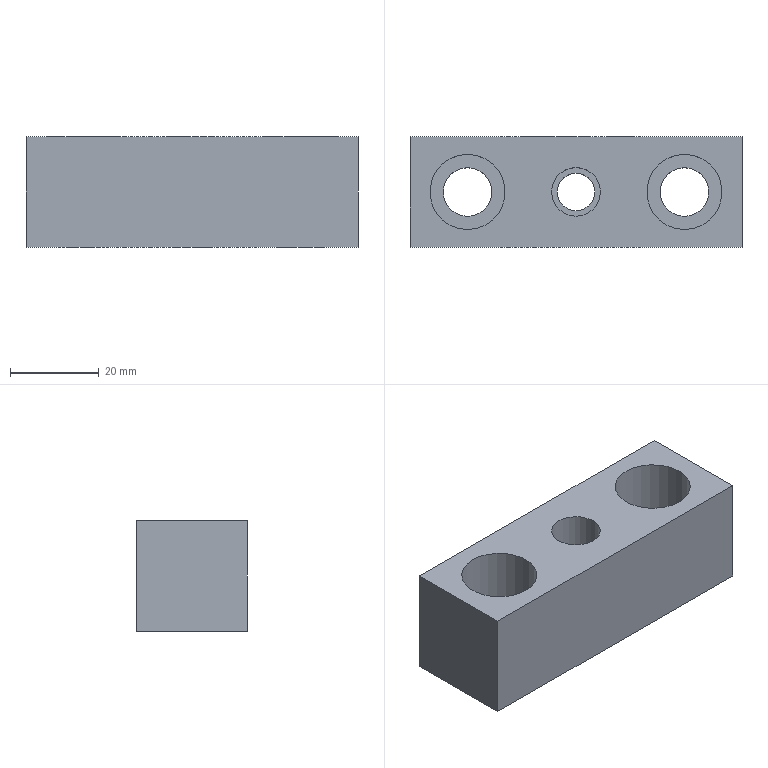Part | STEP file | lll_id4950_x_t | 1 solid | 85 faces | box 75 x 25 x 25 mm | volume 37034 mm3 | plane 66 | other 13 | cylinder 6 | commonest cylinder face diameters 11 x3 17 x2 8.5 x1